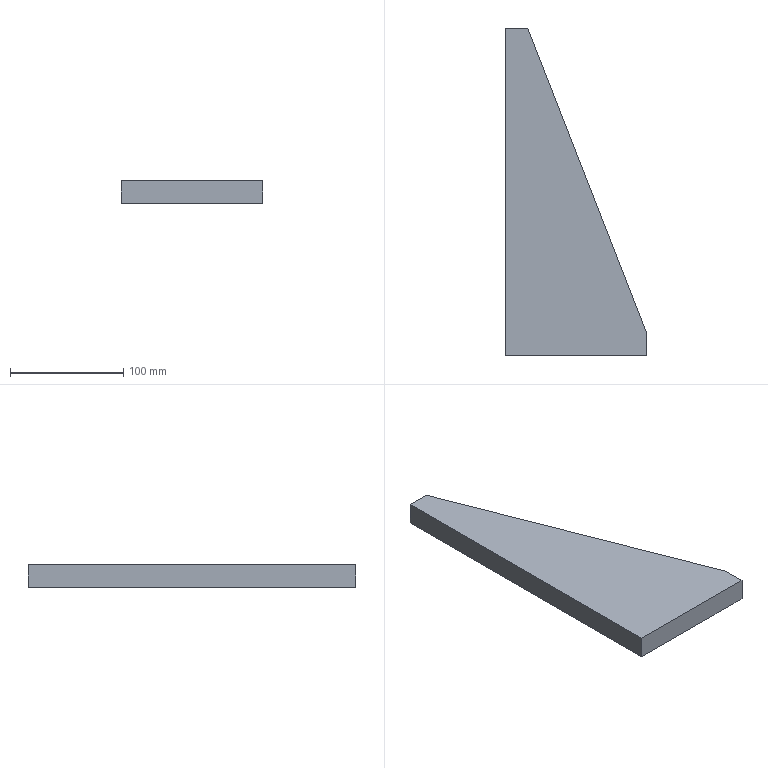Part | SolidWorks | features Extrusion 1 | 1 solid | 7 faces | box 125 x 289 x 20 mm | volume 440050 mm3 | plane 7
STEP:
#1=CARTESIAN_POINT('',(0.,0.,0.));
#2=VERTEX_POINT('',#1);
#3=CARTESIAN_POINT('',(125.,0.,0.));
#4=VERTEX_POINT('',#3);
#5=CARTESIAN_POINT('',(125.,0.,0.));
#6=DIRECTION('',(1.,0.,0.));
#7=VECTOR('',#6,1000.);
#8=LINE('',#5,#7);
#9=EDGE_CURVE('',#2,#4,#8,.T.);
#10=ORIENTED_EDGE('',*,*,#9,.T.);
#11=CARTESIAN_POINT('',(125.,0.,20.));
#12=VERTEX_POINT('',#11);
#13=CARTESIAN_POINT('',(125.,0.,20.));
#14=DIRECTION('',(0.,0.,-1.));
#15=VECTOR('',#14,1000.);
#16=LINE('',#13,#15);
#17=EDGE_CURVE('',#12,#4,#16,.T.);
#18=ORIENTED_EDGE('',*,*,#17,.F.);
#19=CARTESIAN_POINT('',(0.,0.,20.));
#20=VERTEX_POINT('',#19);
#21=CARTESIAN_POINT('',(125.,0.,20.));
#22=DIRECTION('',(1.,0.,0.));
#23=VECTOR('',#22,1000.);
#24=LINE('',#21,#23);
#25=EDGE_CURVE('',#20,#12,#24,.T.);
#26=ORIENTED_EDGE('',*,*,#25,.F.);
#27=CARTESIAN_POINT('',(0.,0.,20.));
#28=DIRECTION('',(0.,0.,-1.));
#29=VECTOR('',#28,1000.);
#30=LINE('',#27,#29);
#31=EDGE_CURVE('',#20,#2,#30,.T.);
#32=ORIENTED_EDGE('',*,*,#31,.T.);
#33=EDGE_LOOP('',(#10,#18,#26,#32));
#34=FACE_OUTER_BOUND('',#33,.T.);
#35=CARTESIAN_POINT('',(125.,0.,20.));
#36=DIRECTION('',(0.,1.,0.));
#37=DIRECTION('',(-1.,0.,0.));
#38=AXIS2_PLACEMENT_3D('',#35,#36,#37);
#39=PLANE('',#38);
#40=ADVANCED_FACE('',(#34),#39,.F.);
#41=CARTESIAN_POINT('',(125.,20.,0.));
#42=VERTEX_POINT('',#41);
#43=CARTESIAN_POINT('',(125.,20.,0.));
#44=DIRECTION('',(0.,1.,0.));
#45=VECTOR('',#44,1000.);
#46=LINE('',#43,#45);
#47=EDGE_CURVE('',#4,#42,#46,.T.);
#48=ORIENTED_EDGE('',*,*,#47,.T.);
#49=CARTESIAN_POINT('',(125.,20.,20.));
#50=VERTEX_POINT('',#49);
#51=CARTESIAN_POINT('',(125.,20.,20.));
#52=DIRECTION('',(0.,0.,-1.));
#53=VECTOR('',#52,1000.);
#54=LINE('',#51,#53);
#55=EDGE_CURVE('',#50,#42,#54,.T.);
#56=ORIENTED_EDGE('',*,*,#55,.F.);
#57=CARTESIAN_POINT('',(125.,20.,20.));
#58=DIRECTION('',(0.,1.,0.));
#59=VECTOR('',#58,1000.);
#60=LINE('',#57,#59);
#61=EDGE_CURVE('',#12,#50,#60,.T.);
#62=ORIENTED_EDGE('',*,*,#61,.F.);
#63=ORIENTED_EDGE('',*,*,#17,.T.);
#64=EDGE_LOOP('',(#48,#56,#62,#63));
#65=FACE_OUTER_BOUND('',#64,.T.);
#66=CARTESIAN_POINT('',(125.,20.,20.));
#67=DIRECTION('',(-1.,0.,0.));
#68=DIRECTION('',(0.,0.,1.));
#69=AXIS2_PLACEMENT_3D('',#66,#67,#68);
#70=PLANE('',#69);
#71=ADVANCED_FACE('',(#65),#70,.F.);
#72=CARTESIAN_POINT('',(20.,289.,0.));
#73=VERTEX_POINT('',#72);
#74=CARTESIAN_POINT('',(20.,289.,0.));
#75=DIRECTION('',(-0.3636,0.9315,0.));
#76=VECTOR('',#75,1000.);
#77=LINE('',#74,#76);
#78=EDGE_CURVE('',#42,#73,#77,.T.);
#79=ORIENTED_EDGE('',*,*,#78,.T.);
#80=CARTESIAN_POINT('',(20.,289.,20.));
#81=VERTEX_POINT('',#80);
#82=CARTESIAN_POINT('',(20.,289.,20.));
#83=DIRECTION('',(0.,0.,-1.));
#84=VECTOR('',#83,1000.);
#85=LINE('',#82,#84);
#86=EDGE_CURVE('',#81,#73,#85,.T.);
#87=ORIENTED_EDGE('',*,*,#86,.F.);
#88=CARTESIAN_POINT('',(20.,289.,20.));
#89=DIRECTION('',(-0.3636,0.9315,0.));
#90=VECTOR('',#89,1000.);
#91=LINE('',#88,#90);
#92=EDGE_CURVE('',#50,#81,#91,.T.);
#93=ORIENTED_EDGE('',*,*,#92,.F.);
#94=ORIENTED_EDGE('',*,*,#55,.T.);
#95=EDGE_LOOP('',(#79,#87,#93,#94));
#96=FACE_OUTER_BOUND('',#95,.T.);
#97=CARTESIAN_POINT('',(20.,289.,20.));
#98=DIRECTION('',(-0.9315,-0.3636,0.));
#99=DIRECTION('',(0.3636,-0.9315,0.));
#100=AXIS2_PLACEMENT_3D('',#97,#98,#99);
#101=PLANE('',#100);
#102=ADVANCED_FACE('',(#96),#101,.F.);
#103=CARTESIAN_POINT('',(0.,289.,0.));
#104=VERTEX_POINT('',#103);
#105=CARTESIAN_POINT('',(0.,289.,0.));
#106=DIRECTION('',(-1.,0.,0.));
#107=VECTOR('',#106,1000.);
#108=LINE('',#105,#107);
#109=EDGE_CURVE('',#73,#104,#108,.T.);
#110=ORIENTED_EDGE('',*,*,#109,.T.);
#111=CARTESIAN_POINT('',(0.,289.,20.));
#112=VERTEX_POINT('',#111);
#113=CARTESIAN_POINT('',(0.,289.,20.));
#114=DIRECTION('',(0.,0.,-1.));
#115=VECTOR('',#114,1000.);
#116=LINE('',#113,#115);
#117=EDGE_CURVE('',#112,#104,#116,.T.);
#118=ORIENTED_EDGE('',*,*,#117,.F.);
#119=CARTESIAN_POINT('',(0.,289.,20.));
#120=DIRECTION('',(-1.,0.,0.));
#121=VECTOR('',#120,1000.);
#122=LINE('',#119,#121);
#123=EDGE_CURVE('',#81,#112,#122,.T.);
#124=ORIENTED_EDGE('',*,*,#123,.F.);
#125=ORIENTED_EDGE('',*,*,#86,.T.);
#126=EDGE_LOOP('',(#110,#118,#124,#125));
#127=FACE_OUTER_BOUND('',#126,.T.);
#128=CARTESIAN_POINT('',(0.,289.,20.));
#129=DIRECTION('',(0.,-1.,0.));
#130=DIRECTION('',(0.,0.,-1.));
#131=AXIS2_PLACEMENT_3D('',#128,#129,#130);
#132=PLANE('',#131);
#133=ADVANCED_FACE('',(#127),#132,.F.);
#134=CARTESIAN_POINT('',(0.,0.,0.));
#135=DIRECTION('',(0.,-1.,0.));
#136=VECTOR('',#135,1000.);
#137=LINE('',#134,#136);
#138=EDGE_CURVE('',#104,#2,#137,.T.);
#139=ORIENTED_EDGE('',*,*,#138,.T.);
#140=ORIENTED_EDGE('',*,*,#31,.F.);
#141=CARTESIAN_POINT('',(0.,0.,20.));
#142=DIRECTION('',(0.,-1.,0.));
#143=VECTOR('',#142,1000.);
#144=LINE('',#141,#143);
#145=EDGE_CURVE('',#112,#20,#144,.T.);
#146=ORIENTED_EDGE('',*,*,#145,.F.);
#147=ORIENTED_EDGE('',*,*,#117,.T.);
#148=EDGE_LOOP('',(#139,#140,#146,#147));
#149=FACE_OUTER_BOUND('',#148,.T.);
#150=CARTESIAN_POINT('',(0.,0.,20.));
#151=DIRECTION('',(1.,0.,0.));
#152=DIRECTION('',(0.,0.,-1.));
#153=AXIS2_PLACEMENT_3D('',#150,#151,#152);
#154=PLANE('',#153);
#155=ADVANCED_FACE('',(#149),#154,.F.);
#156=ORIENTED_EDGE('',*,*,#25,.T.);
#157=ORIENTED_EDGE('',*,*,#61,.T.);
#158=ORIENTED_EDGE('',*,*,#92,.T.);
#159=ORIENTED_EDGE('',*,*,#123,.T.);
#160=ORIENTED_EDGE('',*,*,#145,.T.);
#161=EDGE_LOOP('',(#156,#157,#158,#159,#160));
#162=FACE_OUTER_BOUND('',#161,.T.);
#163=CARTESIAN_POINT('',(0.,0.,20.));
#164=DIRECTION('',(0.,0.,-1.));
#165=DIRECTION('',(-1.,0.,0.));
#166=AXIS2_PLACEMENT_3D('',#163,#164,#165);
#167=PLANE('',#166);
#168=ADVANCED_FACE('',(#162),#167,.F.);
#169=ORIENTED_EDGE('',*,*,#9,.F.);
#170=ORIENTED_EDGE('',*,*,#138,.F.);
#171=ORIENTED_EDGE('',*,*,#109,.F.);
#172=ORIENTED_EDGE('',*,*,#78,.F.);
#173=ORIENTED_EDGE('',*,*,#47,.F.);
#174=EDGE_LOOP('',(#169,#170,#171,#172,#173));
#175=FACE_OUTER_BOUND('',#174,.T.);
#176=CARTESIAN_POINT('',(0.,0.,0.));
#177=DIRECTION('',(0.,0.,-1.));
#178=DIRECTION('',(-1.,0.,0.));
#179=AXIS2_PLACEMENT_3D('',#176,#177,#178);
#180=PLANE('',#179);
#181=ADVANCED_FACE('',(#175),#180,.T.);
#182=CLOSED_SHELL('',(#40,#71,#102,#133,#155,#168,#181));
#183=MANIFOLD_SOLID_BREP('',#182);
#184=CARTESIAN_POINT('',(0.,0.,0.));
#185=DIRECTION('',(0.,0.,1.));
#186=DIRECTION('',(1.,0.,0.));
#187=AXIS2_PLACEMENT_3D('',#184,#185,#186);
#188=(LENGTH_UNIT()NAMED_UNIT(*)SI_UNIT(.MILLI.,.METRE.));
#189=UNCERTAINTY_MEASURE_WITH_UNIT(LENGTH_MEASURE(0.00001),#188,'','');
#190=(NAMED_UNIT(*)PLANE_ANGLE_UNIT()SI_UNIT($,.RADIAN.));
#191=(NAMED_UNIT(*)SI_UNIT($,.STERADIAN.)SOLID_ANGLE_UNIT());
#192=(GEOMETRIC_REPRESENTATION_CONTEXT(3)GLOBAL_UNCERTAINTY_ASSIGNED_CONTEXT((#189))GLOBAL_UNIT_ASSIGNED_CONTEXT((#188,#190,#191))REPRESENTATION_CONTEXT('',''));
#193=ADVANCED_BREP_SHAPE_REPRESENTATION('',(#183,#187),#192);